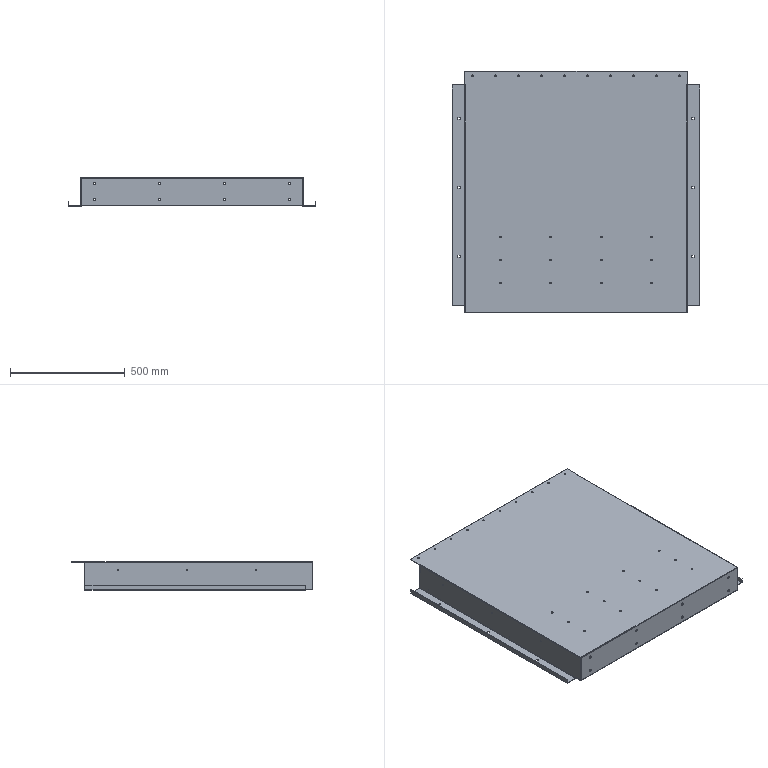Part | STEP file | SX-006-01 | 1 solid | 212 faces | box 1076 x 1051 x 125 mm | volume 3069704 mm3 | cylinder 116 | plane 94 | spline 2 | commonest cylinder face diameters 8 x42 5.4 x22 7 x20 10.5 x16 0.4 x8 4.4 x8